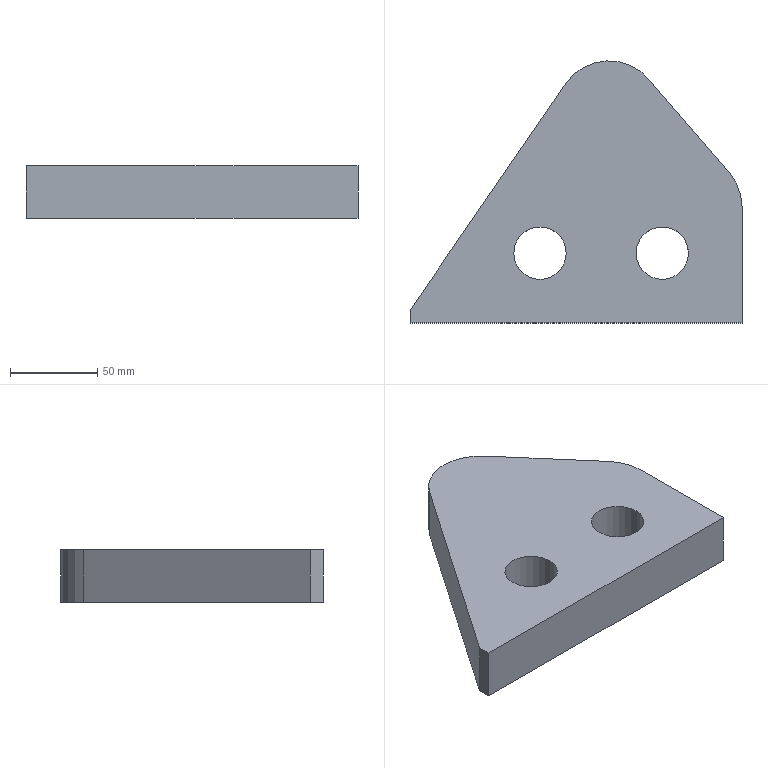Part | SolidWorks | features Extrusion 1 | 1 solid | 13 faces | box 190 x 150.029 x 30 mm | volume 532752 mm3 | plane 7 | cylinder 6 | commonest cylinder face diameters 30 x4 60 x2
STEP:
#1=CARTESIAN_POINT('',(137413.035,-173241.943,30.));
#2=VERTEX_POINT('',#1);
#3=CARTESIAN_POINT('',(137443.035,-173241.943,30.));
#4=VERTEX_POINT('',#3);
#5=CARTESIAN_POINT('',(137428.035,-173241.943,30.));
#6=DIRECTION('',(0.,0.,1.));
#7=DIRECTION('',(1.,0.,0.));
#8=AXIS2_PLACEMENT_3D('',#5,#6,#7);
#9=CIRCLE('',#8,15.);
#10=EDGE_CURVE('',#2,#4,#9,.T.);
#11=ORIENTED_EDGE('',*,*,#10,.T.);
#12=CARTESIAN_POINT('',(137443.035,-173241.943,0.));
#13=VERTEX_POINT('',#12);
#14=CARTESIAN_POINT('',(137443.035,-173241.943,30.));
#15=DIRECTION('',(0.,0.,-1.));
#16=VECTOR('',#15,1000.);
#17=LINE('',#14,#16);
#18=EDGE_CURVE('',#4,#13,#17,.T.);
#19=ORIENTED_EDGE('',*,*,#18,.T.);
#20=CARTESIAN_POINT('',(137413.035,-173241.943,0.));
#21=VERTEX_POINT('',#20);
#22=CARTESIAN_POINT('',(137428.035,-173241.943,0.));
#23=DIRECTION('',(0.,0.,1.));
#24=DIRECTION('',(1.,0.,0.));
#25=AXIS2_PLACEMENT_3D('',#22,#23,#24);
#26=CIRCLE('',#25,15.);
#27=EDGE_CURVE('',#21,#13,#26,.T.);
#28=ORIENTED_EDGE('',*,*,#27,.F.);
#29=CARTESIAN_POINT('',(137413.035,-173241.943,30.));
#30=DIRECTION('',(0.,0.,-1.));
#31=VECTOR('',#30,1000.);
#32=LINE('',#29,#31);
#33=EDGE_CURVE('',#2,#21,#32,.T.);
#34=ORIENTED_EDGE('',*,*,#33,.F.);
#35=EDGE_LOOP('',(#11,#19,#28,#34));
#36=FACE_OUTER_BOUND('',#35,.T.);
#37=CARTESIAN_POINT('',(137428.035,-173241.943,30.));
#38=DIRECTION('',(0.,0.,-1.));
#39=DIRECTION('',(-1.,0.,0.));
#40=AXIS2_PLACEMENT_3D('',#37,#38,#39);
#41=CYLINDRICAL_SURFACE('',#40,15.);
#42=ADVANCED_FACE('',(#36),#41,.F.);
#43=CARTESIAN_POINT('',(137483.035,-173241.943,30.));
#44=VERTEX_POINT('',#43);
#45=CARTESIAN_POINT('',(137513.035,-173241.943,30.));
#46=VERTEX_POINT('',#45);
#47=CARTESIAN_POINT('',(137498.035,-173241.943,30.));
#48=DIRECTION('',(0.,0.,1.));
#49=DIRECTION('',(1.,0.,0.));
#50=AXIS2_PLACEMENT_3D('',#47,#48,#49);
#51=CIRCLE('',#50,15.);
#52=EDGE_CURVE('',#44,#46,#51,.T.);
#53=ORIENTED_EDGE('',*,*,#52,.T.);
#54=CARTESIAN_POINT('',(137513.035,-173241.943,0.));
#55=VERTEX_POINT('',#54);
#56=CARTESIAN_POINT('',(137513.035,-173241.943,30.));
#57=DIRECTION('',(0.,0.,-1.));
#58=VECTOR('',#57,1000.);
#59=LINE('',#56,#58);
#60=EDGE_CURVE('',#46,#55,#59,.T.);
#61=ORIENTED_EDGE('',*,*,#60,.T.);
#62=CARTESIAN_POINT('',(137483.035,-173241.943,0.));
#63=VERTEX_POINT('',#62);
#64=CARTESIAN_POINT('',(137498.035,-173241.943,0.));
#65=DIRECTION('',(0.,0.,1.));
#66=DIRECTION('',(1.,0.,0.));
#67=AXIS2_PLACEMENT_3D('',#64,#65,#66);
#68=CIRCLE('',#67,15.);
#69=EDGE_CURVE('',#63,#55,#68,.T.);
#70=ORIENTED_EDGE('',*,*,#69,.F.);
#71=CARTESIAN_POINT('',(137483.035,-173241.943,30.));
#72=DIRECTION('',(0.,0.,-1.));
#73=VECTOR('',#72,1000.);
#74=LINE('',#71,#73);
#75=EDGE_CURVE('',#44,#63,#74,.T.);
#76=ORIENTED_EDGE('',*,*,#75,.F.);
#77=EDGE_LOOP('',(#53,#61,#70,#76));
#78=FACE_OUTER_BOUND('',#77,.T.);
#79=CARTESIAN_POINT('',(137498.035,-173241.943,30.));
#80=DIRECTION('',(0.,0.,-1.));
#81=DIRECTION('',(-1.,0.,0.));
#82=AXIS2_PLACEMENT_3D('',#79,#80,#81);
#83=CYLINDRICAL_SURFACE('',#82,15.);
#84=ADVANCED_FACE('',(#78),#83,.F.);
#85=ORIENTED_EDGE('',*,*,#52,.F.);
#86=CARTESIAN_POINT('',(137498.035,-173241.943,30.));
#87=DIRECTION('',(0.,0.,1.));
#88=DIRECTION('',(1.,0.,0.));
#89=AXIS2_PLACEMENT_3D('',#86,#87,#88);
#90=CIRCLE('',#89,15.);
#91=EDGE_CURVE('',#46,#44,#90,.T.);
#92=ORIENTED_EDGE('',*,*,#91,.F.);
#93=EDGE_LOOP('',(#85,#92));
#94=FACE_BOUND('',#93,.T.);
#95=CARTESIAN_POINT('',(137490.25,-173142.343,30.));
#96=VERTEX_POINT('',#95);
#97=CARTESIAN_POINT('',(137442.792,-173144.918,30.));
#98=VERTEX_POINT('',#97);
#99=CARTESIAN_POINT('',(137467.513,-173161.914,30.));
#100=DIRECTION('',(0.,0.,1.));
#101=DIRECTION('',(1.,0.,0.));
#102=AXIS2_PLACEMENT_3D('',#99,#100,#101);
#103=CIRCLE('',#102,30.);
#104=EDGE_CURVE('',#96,#98,#103,.T.);
#105=ORIENTED_EDGE('',*,*,#104,.T.);
#106=CARTESIAN_POINT('',(137353.66,-173274.566,30.));
#107=VERTEX_POINT('',#106);
#108=CARTESIAN_POINT('',(137442.792,-173144.918,30.));
#109=DIRECTION('',(-0.5665,-0.824,0.));
#110=VECTOR('',#109,1000.);
#111=LINE('',#108,#110);
#112=EDGE_CURVE('',#98,#107,#111,.T.);
#113=ORIENTED_EDGE('',*,*,#112,.T.);
#114=CARTESIAN_POINT('',(137353.66,-173281.943,30.));
#115=VERTEX_POINT('',#114);
#116=CARTESIAN_POINT('',(137353.66,-173274.566,30.));
#117=DIRECTION('',(0.,-1.,0.));
#118=VECTOR('',#117,1000.);
#119=LINE('',#116,#118);
#120=EDGE_CURVE('',#107,#115,#119,.T.);
#121=ORIENTED_EDGE('',*,*,#120,.T.);
#122=CARTESIAN_POINT('',(137543.66,-173281.943,30.));
#123=VERTEX_POINT('',#122);
#124=CARTESIAN_POINT('',(137353.66,-173281.943,30.));
#125=DIRECTION('',(1.,0.,0.));
#126=VECTOR('',#125,1000.);
#127=LINE('',#124,#126);
#128=EDGE_CURVE('',#115,#123,#127,.T.);
#129=ORIENTED_EDGE('',*,*,#128,.T.);
#130=CARTESIAN_POINT('',(137543.66,-173215.524,30.));
#131=VERTEX_POINT('',#130);
#132=CARTESIAN_POINT('',(137543.66,-173281.943,30.));
#133=DIRECTION('',(0.,1.,0.));
#134=VECTOR('',#133,1000.);
#135=LINE('',#132,#134);
#136=EDGE_CURVE('',#123,#131,#135,.T.);
#137=ORIENTED_EDGE('',*,*,#136,.T.);
#138=CARTESIAN_POINT('',(137536.396,-173195.953,30.));
#139=VERTEX_POINT('',#138);
#140=CARTESIAN_POINT('',(137513.66,-173215.524,30.));
#141=DIRECTION('',(0.,0.,1.));
#142=DIRECTION('',(1.,0.,0.));
#143=AXIS2_PLACEMENT_3D('',#140,#141,#142);
#144=CIRCLE('',#143,30.);
#145=EDGE_CURVE('',#131,#139,#144,.T.);
#146=ORIENTED_EDGE('',*,*,#145,.T.);
#147=CARTESIAN_POINT('',(137536.396,-173195.953,30.));
#148=DIRECTION('',(-0.6524,0.7579,0.));
#149=VECTOR('',#148,1000.);
#150=LINE('',#147,#149);
#151=EDGE_CURVE('',#139,#96,#150,.T.);
#152=ORIENTED_EDGE('',*,*,#151,.T.);
#153=EDGE_LOOP('',(#105,#113,#121,#129,#137,#146,#152));
#154=FACE_OUTER_BOUND('',#153,.T.);
#155=ORIENTED_EDGE('',*,*,#10,.F.);
#156=CARTESIAN_POINT('',(137428.035,-173241.943,30.));
#157=DIRECTION('',(0.,0.,1.));
#158=DIRECTION('',(1.,0.,0.));
#159=AXIS2_PLACEMENT_3D('',#156,#157,#158);
#160=CIRCLE('',#159,15.);
#161=EDGE_CURVE('',#4,#2,#160,.T.);
#162=ORIENTED_EDGE('',*,*,#161,.F.);
#163=EDGE_LOOP('',(#155,#162));
#164=FACE_BOUND('',#163,.T.);
#165=CARTESIAN_POINT('',(137467.513,-173161.914,30.));
#166=DIRECTION('',(0.,0.,1.));
#167=DIRECTION('',(1.,0.,0.));
#168=AXIS2_PLACEMENT_3D('',#165,#166,#167);
#169=PLANE('',#168);
#170=ADVANCED_FACE('',(#94,#154,#164),#169,.T.);
#171=CARTESIAN_POINT('',(137490.25,-173142.343,0.));
#172=VERTEX_POINT('',#171);
#173=CARTESIAN_POINT('',(137442.792,-173144.918,0.));
#174=VERTEX_POINT('',#173);
#175=CARTESIAN_POINT('',(137467.513,-173161.914,0.));
#176=DIRECTION('',(0.,0.,1.));
#177=DIRECTION('',(1.,0.,0.));
#178=AXIS2_PLACEMENT_3D('',#175,#176,#177);
#179=CIRCLE('',#178,30.);
#180=EDGE_CURVE('',#172,#174,#179,.T.);
#181=ORIENTED_EDGE('',*,*,#180,.F.);
#182=CARTESIAN_POINT('',(137536.396,-173195.953,0.));
#183=VERTEX_POINT('',#182);
#184=CARTESIAN_POINT('',(137536.396,-173195.953,0.));
#185=DIRECTION('',(-0.6524,0.7579,0.));
#186=VECTOR('',#185,1000.);
#187=LINE('',#184,#186);
#188=EDGE_CURVE('',#183,#172,#187,.T.);
#189=ORIENTED_EDGE('',*,*,#188,.F.);
#190=CARTESIAN_POINT('',(137543.66,-173215.524,0.));
#191=VERTEX_POINT('',#190);
#192=CARTESIAN_POINT('',(137513.66,-173215.524,0.));
#193=DIRECTION('',(0.,0.,1.));
#194=DIRECTION('',(1.,0.,0.));
#195=AXIS2_PLACEMENT_3D('',#192,#193,#194);
#196=CIRCLE('',#195,30.);
#197=EDGE_CURVE('',#191,#183,#196,.T.);
#198=ORIENTED_EDGE('',*,*,#197,.F.);
#199=CARTESIAN_POINT('',(137543.66,-173281.943,0.));
#200=VERTEX_POINT('',#199);
#201=CARTESIAN_POINT('',(137543.66,-173281.943,0.));
#202=DIRECTION('',(0.,1.,0.));
#203=VECTOR('',#202,1000.);
#204=LINE('',#201,#203);
#205=EDGE_CURVE('',#200,#191,#204,.T.);
#206=ORIENTED_EDGE('',*,*,#205,.F.);
#207=CARTESIAN_POINT('',(137353.66,-173281.943,0.));
#208=VERTEX_POINT('',#207);
#209=CARTESIAN_POINT('',(137353.66,-173281.943,0.));
#210=DIRECTION('',(1.,0.,0.));
#211=VECTOR('',#210,1000.);
#212=LINE('',#209,#211);
#213=EDGE_CURVE('',#208,#200,#212,.T.);
#214=ORIENTED_EDGE('',*,*,#213,.F.);
#215=CARTESIAN_POINT('',(137353.66,-173274.566,0.));
#216=VERTEX_POINT('',#215);
#217=CARTESIAN_POINT('',(137353.66,-173274.566,0.));
#218=DIRECTION('',(0.,-1.,0.));
#219=VECTOR('',#218,1000.);
#220=LINE('',#217,#219);
#221=EDGE_CURVE('',#216,#208,#220,.T.);
#222=ORIENTED_EDGE('',*,*,#221,.F.);
#223=CARTESIAN_POINT('',(137442.792,-173144.918,0.));
#224=DIRECTION('',(-0.5665,-0.824,0.));
#225=VECTOR('',#224,1000.);
#226=LINE('',#223,#225);
#227=EDGE_CURVE('',#174,#216,#226,.T.);
#228=ORIENTED_EDGE('',*,*,#227,.F.);
#229=EDGE_LOOP('',(#181,#189,#198,#206,#214,#222,#228));
#230=FACE_OUTER_BOUND('',#229,.T.);
#231=ORIENTED_EDGE('',*,*,#69,.T.);
#232=CARTESIAN_POINT('',(137498.035,-173241.943,0.));
#233=DIRECTION('',(0.,0.,1.));
#234=DIRECTION('',(1.,0.,0.));
#235=AXIS2_PLACEMENT_3D('',#232,#233,#234);
#236=CIRCLE('',#235,15.);
#237=EDGE_CURVE('',#55,#63,#236,.T.);
#238=ORIENTED_EDGE('',*,*,#237,.T.);
#239=EDGE_LOOP('',(#231,#238));
#240=FACE_BOUND('',#239,.T.);
#241=ORIENTED_EDGE('',*,*,#27,.T.);
#242=CARTESIAN_POINT('',(137428.035,-173241.943,0.));
#243=DIRECTION('',(0.,0.,1.));
#244=DIRECTION('',(1.,0.,0.));
#245=AXIS2_PLACEMENT_3D('',#242,#243,#244);
#246=CIRCLE('',#245,15.);
#247=EDGE_CURVE('',#13,#21,#246,.T.);
#248=ORIENTED_EDGE('',*,*,#247,.T.);
#249=EDGE_LOOP('',(#241,#248));
#250=FACE_BOUND('',#249,.T.);
#251=CARTESIAN_POINT('',(137467.513,-173161.914,0.));
#252=DIRECTION('',(0.,0.,1.));
#253=DIRECTION('',(1.,0.,0.));
#254=AXIS2_PLACEMENT_3D('',#251,#252,#253);
#255=PLANE('',#254);
#256=ADVANCED_FACE('',(#230,#240,#250),#255,.F.);
#257=ORIENTED_EDGE('',*,*,#180,.T.);
#258=CARTESIAN_POINT('',(137442.792,-173144.918,30.));
#259=DIRECTION('',(0.,0.,-1.));
#260=VECTOR('',#259,1000.);
#261=LINE('',#258,#260);
#262=EDGE_CURVE('',#98,#174,#261,.T.);
#263=ORIENTED_EDGE('',*,*,#262,.F.);
#264=ORIENTED_EDGE('',*,*,#104,.F.);
#265=CARTESIAN_POINT('',(137490.25,-173142.343,30.));
#266=DIRECTION('',(0.,0.,-1.));
#267=VECTOR('',#266,1000.);
#268=LINE('',#265,#267);
#269=EDGE_CURVE('',#96,#172,#268,.T.);
#270=ORIENTED_EDGE('',*,*,#269,.T.);
#271=EDGE_LOOP('',(#257,#263,#264,#270));
#272=FACE_OUTER_BOUND('',#271,.T.);
#273=CARTESIAN_POINT('',(137467.513,-173161.914,30.));
#274=DIRECTION('',(0.,0.,-1.));
#275=DIRECTION('',(-1.,0.,0.));
#276=AXIS2_PLACEMENT_3D('',#273,#274,#275);
#277=CYLINDRICAL_SURFACE('',#276,30.);
#278=ADVANCED_FACE('',(#272),#277,.T.);
#279=ORIENTED_EDGE('',*,*,#227,.T.);
#280=CARTESIAN_POINT('',(137353.66,-173274.566,30.));
#281=DIRECTION('',(0.,0.,-1.));
#282=VECTOR('',#281,1000.);
#283=LINE('',#280,#282);
#284=EDGE_CURVE('',#107,#216,#283,.T.);
#285=ORIENTED_EDGE('',*,*,#284,.F.);
#286=ORIENTED_EDGE('',*,*,#112,.F.);
#287=ORIENTED_EDGE('',*,*,#262,.T.);
#288=EDGE_LOOP('',(#279,#285,#286,#287));
#289=FACE_OUTER_BOUND('',#288,.T.);
#290=CARTESIAN_POINT('',(137442.792,-173144.918,30.));
#291=DIRECTION('',(0.824,-0.5665,0.));
#292=DIRECTION('',(0.5665,0.824,0.));
#293=AXIS2_PLACEMENT_3D('',#290,#291,#292);
#294=PLANE('',#293);
#295=ADVANCED_FACE('',(#289),#294,.F.);
#296=ORIENTED_EDGE('',*,*,#221,.T.);
#297=CARTESIAN_POINT('',(137353.66,-173281.943,30.));
#298=DIRECTION('',(0.,0.,-1.));
#299=VECTOR('',#298,1000.);
#300=LINE('',#297,#299);
#301=EDGE_CURVE('',#115,#208,#300,.T.);
#302=ORIENTED_EDGE('',*,*,#301,.F.);
#303=ORIENTED_EDGE('',*,*,#120,.F.);
#304=ORIENTED_EDGE('',*,*,#284,.T.);
#305=EDGE_LOOP('',(#296,#302,#303,#304));
#306=FACE_OUTER_BOUND('',#305,.T.);
#307=CARTESIAN_POINT('',(137353.66,-173274.566,30.));
#308=DIRECTION('',(1.,0.,0.));
#309=DIRECTION('',(0.,0.,-1.));
#310=AXIS2_PLACEMENT_3D('',#307,#308,#309);
#311=PLANE('',#310);
#312=ADVANCED_FACE('',(#306),#311,.F.);
#313=ORIENTED_EDGE('',*,*,#213,.T.);
#314=CARTESIAN_POINT('',(137543.66,-173281.943,30.));
#315=DIRECTION('',(0.,0.,-1.));
#316=VECTOR('',#315,1000.);
#317=LINE('',#314,#316);
#318=EDGE_CURVE('',#123,#200,#317,.T.);
#319=ORIENTED_EDGE('',*,*,#318,.F.);
#320=ORIENTED_EDGE('',*,*,#128,.F.);
#321=ORIENTED_EDGE('',*,*,#301,.T.);
#322=EDGE_LOOP('',(#313,#319,#320,#321));
#323=FACE_OUTER_BOUND('',#322,.T.);
#324=CARTESIAN_POINT('',(137353.66,-173281.943,30.));
#325=DIRECTION('',(0.,1.,0.));
#326=DIRECTION('',(0.,0.,1.));
#327=AXIS2_PLACEMENT_3D('',#324,#325,#326);
#328=PLANE('',#327);
#329=ADVANCED_FACE('',(#323),#328,.F.);
#330=ORIENTED_EDGE('',*,*,#205,.T.);
#331=CARTESIAN_POINT('',(137543.66,-173215.524,30.));
#332=DIRECTION('',(0.,0.,-1.));
#333=VECTOR('',#332,1000.);
#334=LINE('',#331,#333);
#335=EDGE_CURVE('',#131,#191,#334,.T.);
#336=ORIENTED_EDGE('',*,*,#335,.F.);
#337=ORIENTED_EDGE('',*,*,#136,.F.);
#338=ORIENTED_EDGE('',*,*,#318,.T.);
#339=EDGE_LOOP('',(#330,#336,#337,#338));
#340=FACE_OUTER_BOUND('',#339,.T.);
#341=CARTESIAN_POINT('',(137543.66,-173281.943,30.));
#342=DIRECTION('',(-1.,0.,0.));
#343=DIRECTION('',(0.,0.,1.));
#344=AXIS2_PLACEMENT_3D('',#341,#342,#343);
#345=PLANE('',#344);
#346=ADVANCED_FACE('',(#340),#345,.F.);
#347=ORIENTED_EDGE('',*,*,#197,.T.);
#348=CARTESIAN_POINT('',(137536.396,-173195.953,30.));
#349=DIRECTION('',(0.,0.,-1.));
#350=VECTOR('',#349,1000.);
#351=LINE('',#348,#350);
#352=EDGE_CURVE('',#139,#183,#351,.T.);
#353=ORIENTED_EDGE('',*,*,#352,.F.);
#354=ORIENTED_EDGE('',*,*,#145,.F.);
#355=ORIENTED_EDGE('',*,*,#335,.T.);
#356=EDGE_LOOP('',(#347,#353,#354,#355));
#357=FACE_OUTER_BOUND('',#356,.T.);
#358=CARTESIAN_POINT('',(137513.66,-173215.524,30.));
#359=DIRECTION('',(0.,0.,-1.));
#360=DIRECTION('',(-1.,0.,0.));
#361=AXIS2_PLACEMENT_3D('',#358,#359,#360);
#362=CYLINDRICAL_SURFACE('',#361,30.);
#363=ADVANCED_FACE('',(#357),#362,.T.);
#364=ORIENTED_EDGE('',*,*,#188,.T.);
#365=ORIENTED_EDGE('',*,*,#269,.F.);
#366=ORIENTED_EDGE('',*,*,#151,.F.);
#367=ORIENTED_EDGE('',*,*,#352,.T.);
#368=EDGE_LOOP('',(#364,#365,#366,#367));
#369=FACE_OUTER_BOUND('',#368,.T.);
#370=CARTESIAN_POINT('',(137536.396,-173195.953,30.));
#371=DIRECTION('',(-0.7579,-0.6524,0.));
#372=DIRECTION('',(0.6524,-0.7579,0.));
#373=AXIS2_PLACEMENT_3D('',#370,#371,#372);
#374=PLANE('',#373);
#375=ADVANCED_FACE('',(#369),#374,.F.);
#376=ORIENTED_EDGE('',*,*,#60,.F.);
#377=ORIENTED_EDGE('',*,*,#91,.T.);
#378=ORIENTED_EDGE('',*,*,#75,.T.);
#379=ORIENTED_EDGE('',*,*,#237,.F.);
#380=EDGE_LOOP('',(#376,#377,#378,#379));
#381=FACE_OUTER_BOUND('',#380,.T.);
#382=CARTESIAN_POINT('',(137498.035,-173241.943,30.));
#383=DIRECTION('',(0.,0.,-1.));
#384=DIRECTION('',(-1.,0.,0.));
#385=AXIS2_PLACEMENT_3D('',#382,#383,#384);
#386=CYLINDRICAL_SURFACE('',#385,15.);
#387=ADVANCED_FACE('',(#381),#386,.F.);
#388=ORIENTED_EDGE('',*,*,#18,.F.);
#389=ORIENTED_EDGE('',*,*,#161,.T.);
#390=ORIENTED_EDGE('',*,*,#33,.T.);
#391=ORIENTED_EDGE('',*,*,#247,.F.);
#392=EDGE_LOOP('',(#388,#389,#390,#391));
#393=FACE_OUTER_BOUND('',#392,.T.);
#394=CARTESIAN_POINT('',(137428.035,-173241.943,30.));
#395=DIRECTION('',(0.,0.,-1.));
#396=DIRECTION('',(-1.,0.,0.));
#397=AXIS2_PLACEMENT_3D('',#394,#395,#396);
#398=CYLINDRICAL_SURFACE('',#397,15.);
#399=ADVANCED_FACE('',(#393),#398,.F.);
#400=CLOSED_SHELL('',(#42,#84,#170,#256,#278,#295,#312,#329,#346,#363,#375,#387,#399));
#401=MANIFOLD_SOLID_BREP('',#400);
#402=CARTESIAN_POINT('',(0.,0.,0.));
#403=DIRECTION('',(0.,0.,1.));
#404=DIRECTION('',(1.,0.,0.));
#405=AXIS2_PLACEMENT_3D('',#402,#403,#404);
#406=(LENGTH_UNIT()NAMED_UNIT(*)SI_UNIT(.MILLI.,.METRE.));
#407=UNCERTAINTY_MEASURE_WITH_UNIT(LENGTH_MEASURE(0.00001),#406,'','');
#408=(NAMED_UNIT(*)PLANE_ANGLE_UNIT()SI_UNIT($,.RADIAN.));
#409=(NAMED_UNIT(*)SI_UNIT($,.STERADIAN.)SOLID_ANGLE_UNIT());
#410=(GEOMETRIC_REPRESENTATION_CONTEXT(3)GLOBAL_UNCERTAINTY_ASSIGNED_CONTEXT((#407))GLOBAL_UNIT_ASSIGNED_CONTEXT((#406,#408,#409))REPRESENTATION_CONTEXT('',''));
#411=ADVANCED_BREP_SHAPE_REPRESENTATION('',(#401,#405),#410);